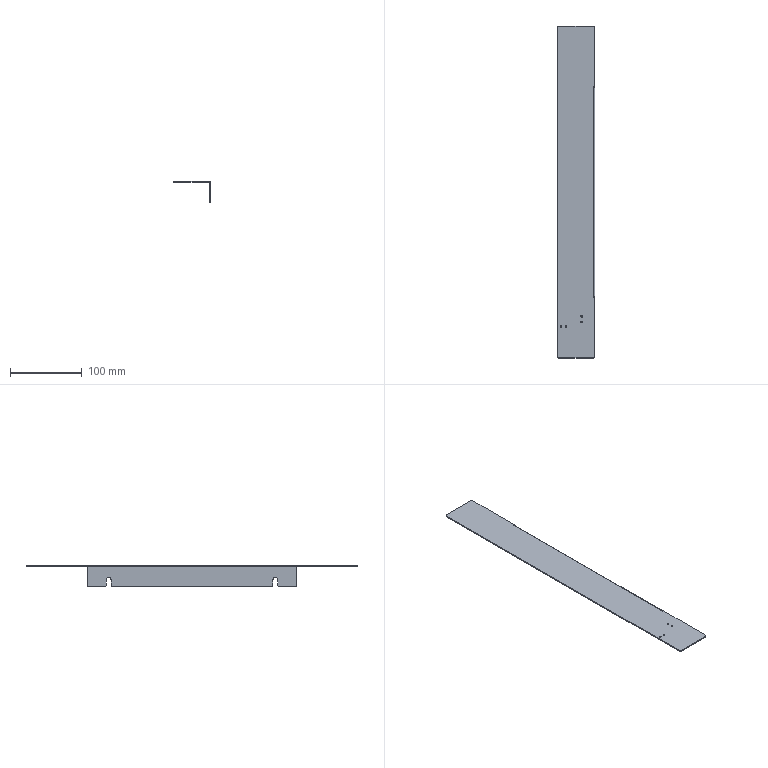Part | STEP file | Lower support plate 2 | 1 solid | 50 faces | box 52 x 462 x 30 mm | volume 48079 mm3 | plane 26 | cylinder 24 | commonest cylinder face diameters 4 x10 2.5 x8 6.6 x4 0.02 x1 3.02 x1